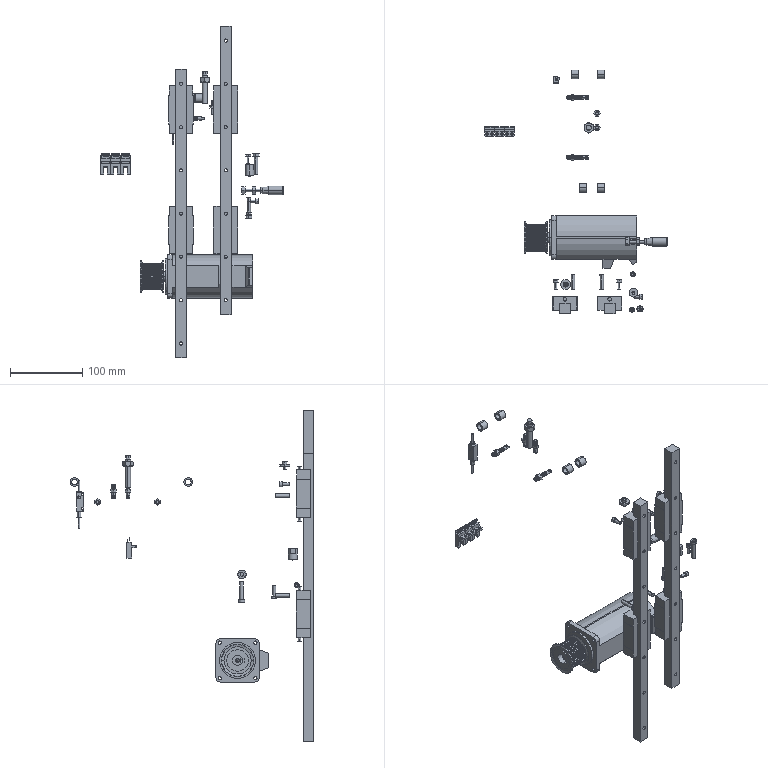Part | NX | 45 solids | 2676 faces | box 253.4 x 337.6 x 460 mm | volume 730030 mm3 | plane 1757 | cylinder 725 | cone 140 | spline 44 | sphere 6 | torus 4 | commonest cylinder face diameters 5 x203 0.5 x52 6.55 x52 1.1 x48 37.24 x48 4.5 x36